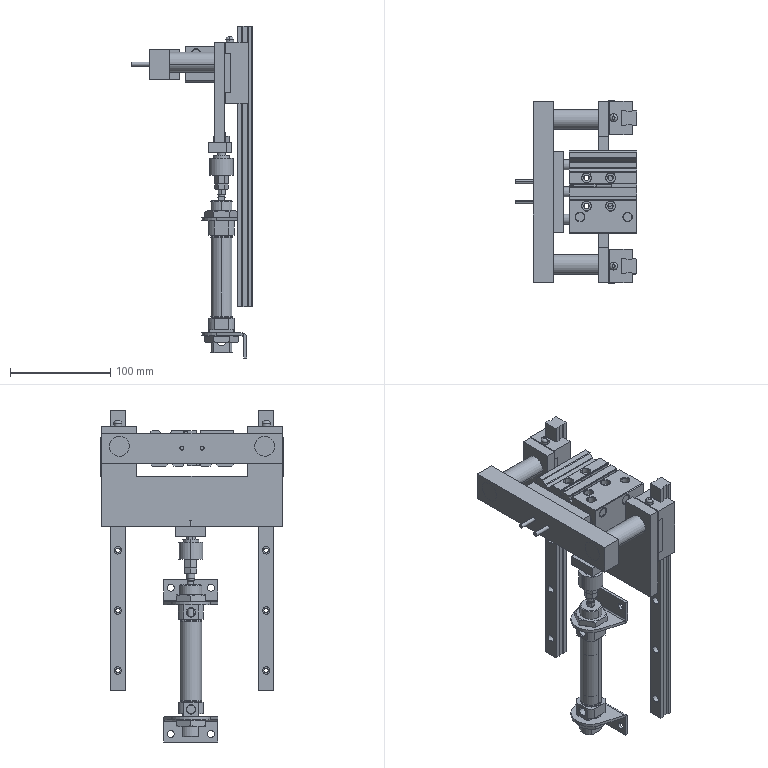Part | SolidWorks | 25 solids | 935 faces | box 121 x 182 x 331.393 mm | volume 727155 mm3 | plane 408 | cylinder 355 | cone 162 | torus 10 | commonest cylinder face diameters 3 x27 0.8 x20 4.5 x20 7.5 x20 0.4 x16 3.2 x16